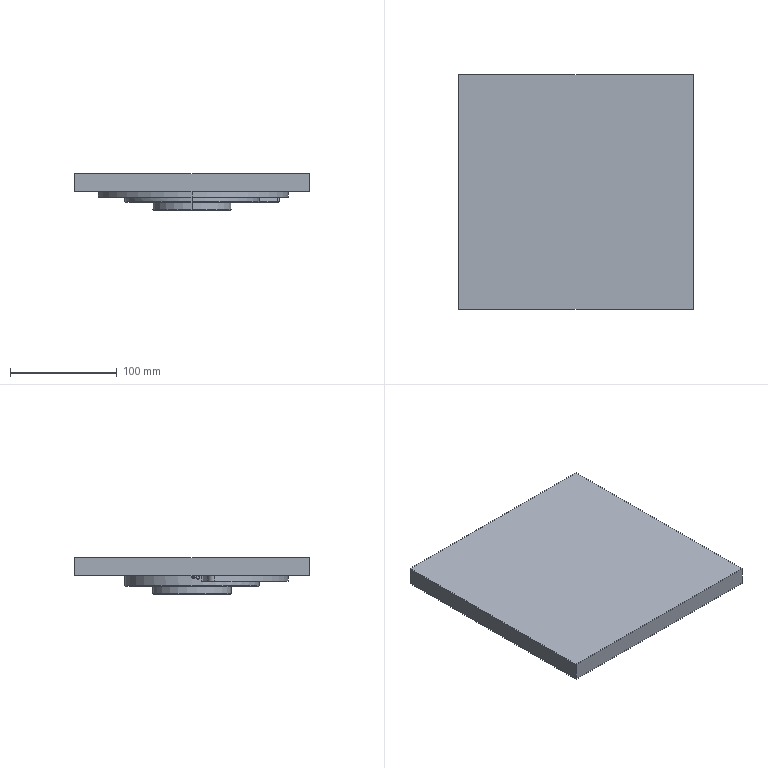CAM job | NX | 3-axis milling, drilling | part box 220 x 220 x 34.5 mm
Tools:
number,name,description,diameter,corner_radius,flute_length,length,flutes
18,D6A45,Milling Tool-5 Parameters,6.0,0.0,3.0,3.0,2
12,2.6ZT,Drilling Tool,2.5,0.0,35.0,50.0,2
13,M3,Milling Tool-5 Parameters,2.5,0.0,30.0,30.0,4
15,5.2ZT,Drilling Tool,5.0,0.0,35.0,50.0,2
16,M6,Milling Tool-5 Parameters,5.0,0.0,30.0,30.0,4
14,4.5ZT,Drilling Tool,4.5,0.0,35.0,50.0,2
3,D10,Milling Tool-5 Parameters,10.0,0.0,50.0,75.0,2
7,D10JING,Milling Tool-5 Parameters,10.0,0.0,50.0,75.0,2
9,D6,Milling Tool-5 Parameters,6.0,0.0,50.0,75.0,2
10,D4,Milling Tool-5 Parameters,4.0,0.0,50.0,75.0,2
20,D2,Milling Tool-5 Parameters,2.0,0.0,50.0,75.0,2
22,D0.5,Milling Tool-5 Parameters,0.5,0.0,50.0,75.0,2
17,3.5ZT,Drilling Tool,3.5,0.0,35.0,50.0,2
Operations:
program,operation,operation_type,tool,method,geometry_group,spindle_rpm,surface_speed,feed_per_tooth,feed_cut,feed_plunge,cut_length_mm,path_length_mm,cut_time_min,machine_time_min
1,DRILLING_COPY_1,Operation,D6A45,METHOD,A,3000.0,56.0,0.0333,200.0,0.0,9.1,91.64,0.0455,0.0538
1,DRILLING_COPY_1_COPY,Operation,D6A45,METHOD,A,3000.0,56.0,0.0333,200.0,0.0,39.2,403.146,0.196,0.2324
1,DRILLING_COPY_1_COPY_1,Operation,2.6ZT,METHOD,A,3000.0,56.0,0.0333,120.0,0.0,22.502,118.445,0.1875,0.1971
1,DRILLING_COPY_1_COPY_1_COPY,Operation,M3,METHOD,A,200.0,1.0,0.0006,0.5,0.0,18.0,109.44,36.0,36.009
1,DRILLING_COPY_1_COPY_1_COPY_1,Operation,5.2ZT,METHOD,A,3000.0,56.0,0.0333,300.0,0.0,108.013,524.219,0.36,0.4017
1,DRILLING_COPY_1_COPY_1_COPY_1_COPY_2,Operation,5.2ZT,METHOD,A,3000.0,56.0,0.0333,300.0,0.0,23.002,106.004,0.0767,0.085
1,DRILLING_COPY_1_COPY_1_COPY_1_COPY,Operation,M6,METHOD,A,200.0,3.0,0.0013,1.0,0.0,93.0,494.193,93.0,93.04
1,DRILLING_COPY_1_COPY_1_COPY_1_COPY_1,Operation,4.5ZT,METHOD,A,3000.0,56.0,0.0333,300.0,0.0,12.852,105.704,0.0428,0.0521
1,ADAPTIVE_MILLING,CavityMilling,D10,METHOD,A,8000.0,251.0,0.2188,3500.0,1000.0,14048.339,20864.329,4.598,5.279
1,ZLEVEL_PROFILE_COPY,ZLevelMilling,D10JING,METHOD,A,8000.0,251.0,0.075,1200.0,100.0,252.092,346.092,0.2101,0.2195
1,ZLEVEL_PROFILE_COPY_1,ZLevelMilling,D6,METHOD,A,9500.0,179.0,0.0789,1500.0,1000.0,1110.017,2314.944,0.8248,0.9453
1,FLOOR_WALL,VolumeBased25DMillingOperation,D6,METHOD,A,9500.0,298.0,0.0526,1000.0,100.0,1294.135,1371.135,1.294,1.302
1,HOLE_MILLING,CylinderMilling,D6,METHOD,A,9500.0,119.0,0.0684,1300.0,100.0,470.696,735.899,0.3621,0.3886
1,ZLEVEL_PROFILE_COPY_1_COPY,ZLevelMilling,D4,METHOD,A,9500.0,179.0,0.0789,1500.0,1000.0,637.476,1237.188,0.4572,0.5172
1,ZLEVEL_PROFILE_COPY_1_COPY_COPY_COPY_COPY_2_COPY,ZLevelMilling,D6A45,METHOD,A,7000.0,131.0,0.0714,1000.0,1000.0,961.618,1265.515,0.9616,0.992
1,ZLEVEL_PROFILE_COPY_2,ZLevelMilling,D2,METHOD,MCS_MILL-A,9500.0,59.0,0.0632,1200.0,1000.0,361.925,416.748,0.3065,0.312
1,ZLEVEL_PROFILE_COPY_2_COPY,ZLevelMilling,D2,METHOD,MCS_MILL-A,9500.0,59.0,0.0632,1200.0,1000.0,249.156,307.158,0.2126,0.2184
1,ZLEVEL_PROFILE_COPY_2_COPY_COPY,ZLevelMilling,D0.5,METHOD,MCS_MILL-A,9500.0,14.0,0.0526,1000.0,1000.0,1861.678,2094.537,1.862,1.885
1,CUTTERCOMP9,CylinderMilling,D6,METHOD,A,9500.0,119.0,0.0447,850.0,100.0,118.453,383.657,0.1394,0.1659
2_FIXTURE,ADAPTIVE_MILLING_COPY,CavityMilling,D10,METHOD,B,8000.0,251.0,0.2188,3500.0,1000.0,24834.315,24895.165,7.499,7.505
2_FIXTURE,FLOOR_WALL_COPY,VolumeBased25DMillingOperation,D10JING,METHOD,B,9500.0,298.0,0.0526,1000.0,100.0,3633.077,3704.077,3.633,3.64
2_FIXTURE,ZLEVEL_PROFILE_COPY_1_COPY_COPY_COPY_COPY_2_COPY_COPY,ZLevelMilling,D6A45,METHOD,B,7000.0,131.0,0.0714,1000.0,1000.0,535.019,597.019,0.535,0.5412
2_FIXTURE,CUTTERCOMP7,VolumeBased25DMillingOperation,D10JING,METHOD,B,9500.0,298.0,0.0526,1000.0,100.0,514.207,585.207,0.5142,0.5213
3,ADAPTIVE_MILLING_COPY_COPY,CavityMilling,D10,METHOD,C,8000.0,251.0,0.2188,3500.0,1000.0,19531.826,19841.129,5.904,5.935
3,ADAPTIVE_MILLING_COPY_COPY_COPY,CavityMilling,D10,METHOD,C,8000.0,251.0,0.2188,3500.0,1000.0,3950.289,4029.139,1.655,1.663
3,FLOOR_WALL_COPY_COPY,VolumeBased25DMillingOperation,D10JING,METHOD,C,9500.0,298.0,0.0526,1000.0,100.0,2366.286,2776.222,2.366,2.407
3,DRILLING_COPY_1_COPY_2,Operation,D6A45,METHOD,C,3000.0,56.0,0.0333,200.0,0.0,13.65,206.043,0.0683,0.0875
3,DRILLING_COPY_1_COPY_2_COPY,Operation,D6A45,METHOD,C,3000.0,56.0,0.0333,200.0,0.0,29.1,266.546,0.1455,0.1692
3,DRILLING_COPY_1_COPY_1_COPY_2,Operation,2.6ZT,METHOD,C,3000.0,56.0,0.0333,120.0,0.0,33.753,246.25,0.2813,0.3025
3,DRILLING_COPY_1_COPY_1_COPY_COPY,Operation,M3,METHOD,C,200.0,1.0,0.0006,0.5,0.0,27.0,232.743,54.0,54.021
3,DRILLING_COPY_1_COPY_1_COPY_2_COPY,Operation,3.5ZT,METHOD,C,3000.0,56.0,0.0333,120.0,0.0,57.309,322.964,0.4776,0.5041
3,ZLEVEL_PROFILE_COPY_1_COPY_COPY_COPY_COPY_2_COPY_COPY_COPY,ZLevelMilling,D6A45,METHOD,C,7000.0,131.0,0.0714,1000.0,1000.0,721.338,1290.831,0.7213,0.7783
3,ZLEVEL_PROFILE_COPY_1_COPY_COPY_COPY_COPY_2_COPY_COPY_COPY_COPY,ZLevelMilling,D6A45,METHOD,C,7000.0,131.0,0.0714,1000.0,1000.0,429.135,1594.534,0.4291,0.5457